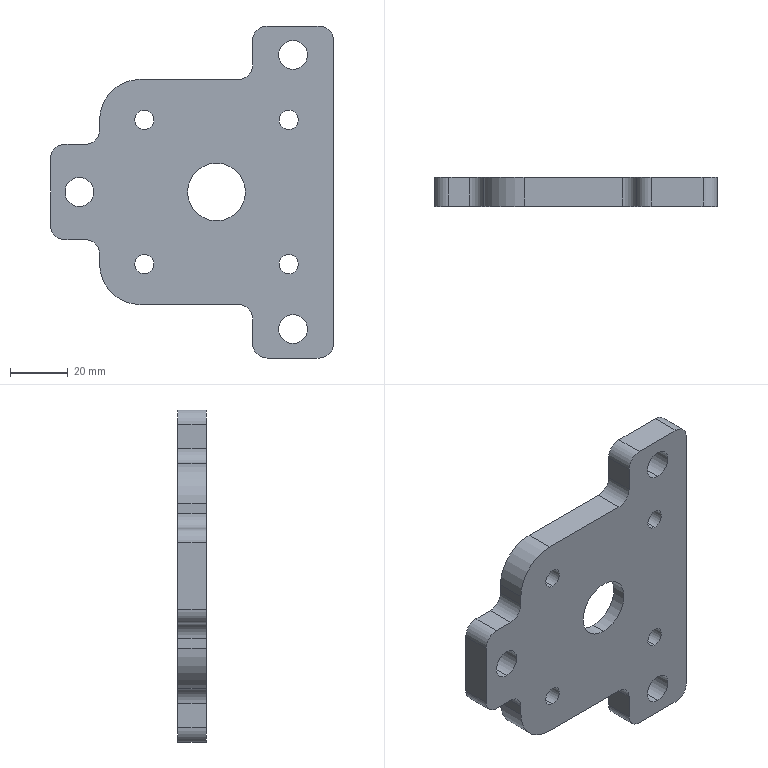Part | SolidWorks | features ICE 5, Fillet 4, Cut 1, Extrusion 1 | 1 solid | 55 faces | box 98 x 10 x 115 mm | volume 49580 mm3 | cylinder 35 | plane 20 | commonest cylinder face diameters 10 x19 6.647 x8 18 x4 20 x2 28 x2